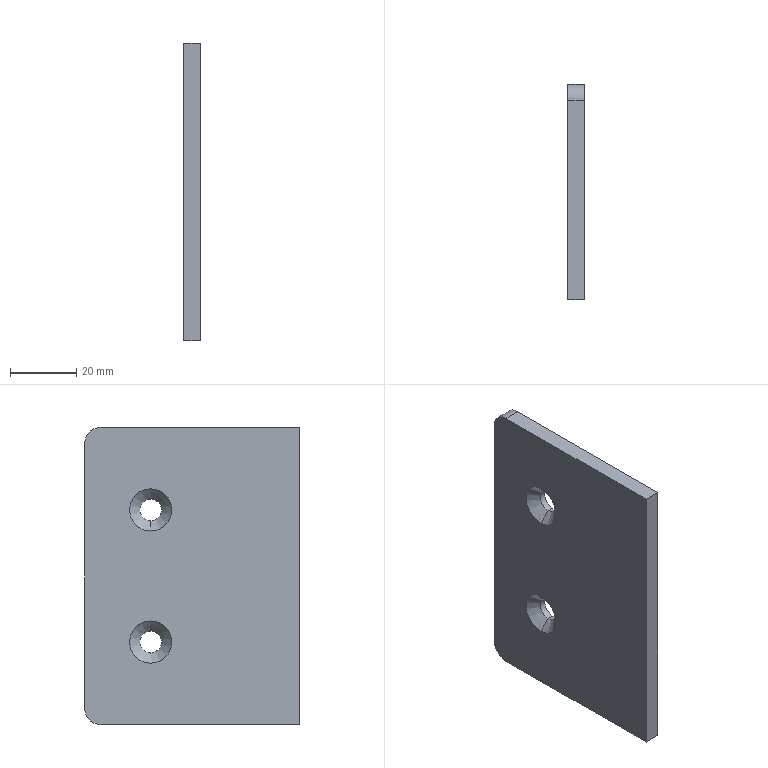Part | SolidWorks | features Extrusion 1, HoleWzd 1 | 1 solid | 16 faces | box 5 x 65 x 90 mm | volume 28593 mm3 | cylinder 6 | plane 6 | cone 4 | commonest cylinder face diameters 6.6 x4 10 x2
STEP:
#1=CARTESIAN_POINT('',(3.1,45.,-23.3));
#2=VERTEX_POINT('',#1);
#3=CARTESIAN_POINT('',(3.1,45.,-16.7));
#4=VERTEX_POINT('',#3);
#5=CARTESIAN_POINT('',(3.1,45.,-20.));
#6=DIRECTION('',(-1.,0.,0.));
#7=DIRECTION('',(0.,0.,1.));
#8=AXIS2_PLACEMENT_3D('',#5,#6,#7);
#9=CIRCLE('',#8,3.3);
#10=EDGE_CURVE('',#2,#4,#9,.T.);
#11=ORIENTED_EDGE('',*,*,#10,.F.);
#12=CARTESIAN_POINT('',(0.,45.,-26.4));
#13=VERTEX_POINT('',#12);
#14=CARTESIAN_POINT('',(0.,45.,-26.4));
#15=DIRECTION('',(-0.7071,0.,-0.7071));
#16=VECTOR('',#15,1000.);
#17=LINE('',#14,#16);
#18=EDGE_CURVE('',#2,#13,#17,.T.);
#19=ORIENTED_EDGE('',*,*,#18,.T.);
#20=CARTESIAN_POINT('',(0.,45.,-13.6));
#21=VERTEX_POINT('',#20);
#22=CARTESIAN_POINT('',(0.,45.,-20.));
#23=DIRECTION('',(-1.,0.,0.));
#24=DIRECTION('',(0.,0.,1.));
#25=AXIS2_PLACEMENT_3D('',#22,#23,#24);
#26=CIRCLE('',#25,6.4);
#27=EDGE_CURVE('',#13,#21,#26,.T.);
#28=ORIENTED_EDGE('',*,*,#27,.T.);
#29=CARTESIAN_POINT('',(0.,45.,-13.6));
#30=DIRECTION('',(-0.7071,0.,0.7071));
#31=VECTOR('',#30,1000.);
#32=LINE('',#29,#31);
#33=EDGE_CURVE('',#4,#21,#32,.T.);
#34=ORIENTED_EDGE('',*,*,#33,.F.);
#35=EDGE_LOOP('',(#11,#19,#28,#34));
#36=FACE_OUTER_BOUND('',#35,.T.);
#37=CARTESIAN_POINT('',(0.,45.,-20.));
#38=DIRECTION('',(-1.,0.,0.));
#39=DIRECTION('',(0.,0.,1.));
#40=AXIS2_PLACEMENT_3D('',#37,#38,#39);
#41=CONICAL_SURFACE('',#40,6.4,0.7854);
#42=ADVANCED_FACE('',(#36),#41,.F.);
#43=CARTESIAN_POINT('',(5.,45.,-23.3));
#44=VERTEX_POINT('',#43);
#45=CARTESIAN_POINT('',(5.,45.,-16.7));
#46=VERTEX_POINT('',#45);
#47=CARTESIAN_POINT('',(5.,45.,-20.));
#48=DIRECTION('',(-1.,0.,0.));
#49=DIRECTION('',(0.,0.,1.));
#50=AXIS2_PLACEMENT_3D('',#47,#48,#49);
#51=CIRCLE('',#50,3.3);
#52=EDGE_CURVE('',#44,#46,#51,.T.);
#53=ORIENTED_EDGE('',*,*,#52,.F.);
#54=CARTESIAN_POINT('',(0.,45.,-23.3));
#55=DIRECTION('',(-1.,0.,0.));
#56=VECTOR('',#55,1000.);
#57=LINE('',#54,#56);
#58=EDGE_CURVE('',#44,#2,#57,.T.);
#59=ORIENTED_EDGE('',*,*,#58,.T.);
#60=ORIENTED_EDGE('',*,*,#10,.T.);
#61=CARTESIAN_POINT('',(0.,45.,-16.7));
#62=DIRECTION('',(-1.,0.,0.));
#63=VECTOR('',#62,1000.);
#64=LINE('',#61,#63);
#65=EDGE_CURVE('',#46,#4,#64,.T.);
#66=ORIENTED_EDGE('',*,*,#65,.F.);
#67=EDGE_LOOP('',(#53,#59,#60,#66));
#68=FACE_OUTER_BOUND('',#67,.T.);
#69=CARTESIAN_POINT('',(0.,45.,-20.));
#70=DIRECTION('',(-1.,0.,0.));
#71=DIRECTION('',(0.,0.,1.));
#72=AXIS2_PLACEMENT_3D('',#69,#70,#71);
#73=CYLINDRICAL_SURFACE('',#72,3.3);
#74=ADVANCED_FACE('',(#68),#73,.F.);
#75=CARTESIAN_POINT('',(3.1,45.,16.7));
#76=VERTEX_POINT('',#75);
#77=CARTESIAN_POINT('',(3.1,45.,23.3));
#78=VERTEX_POINT('',#77);
#79=CARTESIAN_POINT('',(3.1,45.,20.));
#80=DIRECTION('',(-1.,0.,0.));
#81=DIRECTION('',(0.,0.,1.));
#82=AXIS2_PLACEMENT_3D('',#79,#80,#81);
#83=CIRCLE('',#82,3.3);
#84=EDGE_CURVE('',#76,#78,#83,.T.);
#85=ORIENTED_EDGE('',*,*,#84,.F.);
#86=CARTESIAN_POINT('',(0.,45.,13.6));
#87=VERTEX_POINT('',#86);
#88=CARTESIAN_POINT('',(0.,45.,13.6));
#89=DIRECTION('',(-0.7071,0.,-0.7071));
#90=VECTOR('',#89,1000.);
#91=LINE('',#88,#90);
#92=EDGE_CURVE('',#76,#87,#91,.T.);
#93=ORIENTED_EDGE('',*,*,#92,.T.);
#94=CARTESIAN_POINT('',(0.,45.,26.4));
#95=VERTEX_POINT('',#94);
#96=CARTESIAN_POINT('',(0.,45.,20.));
#97=DIRECTION('',(-1.,0.,0.));
#98=DIRECTION('',(0.,0.,1.));
#99=AXIS2_PLACEMENT_3D('',#96,#97,#98);
#100=CIRCLE('',#99,6.4);
#101=EDGE_CURVE('',#87,#95,#100,.T.);
#102=ORIENTED_EDGE('',*,*,#101,.T.);
#103=CARTESIAN_POINT('',(0.,45.,26.4));
#104=DIRECTION('',(-0.7071,0.,0.7071));
#105=VECTOR('',#104,1000.);
#106=LINE('',#103,#105);
#107=EDGE_CURVE('',#78,#95,#106,.T.);
#108=ORIENTED_EDGE('',*,*,#107,.F.);
#109=EDGE_LOOP('',(#85,#93,#102,#108));
#110=FACE_OUTER_BOUND('',#109,.T.);
#111=CARTESIAN_POINT('',(0.,45.,20.));
#112=DIRECTION('',(-1.,0.,0.));
#113=DIRECTION('',(0.,0.,1.));
#114=AXIS2_PLACEMENT_3D('',#111,#112,#113);
#115=CONICAL_SURFACE('',#114,6.4,0.7854);
#116=ADVANCED_FACE('',(#110),#115,.F.);
#117=CARTESIAN_POINT('',(5.,45.,16.7));
#118=VERTEX_POINT('',#117);
#119=CARTESIAN_POINT('',(5.,45.,23.3));
#120=VERTEX_POINT('',#119);
#121=CARTESIAN_POINT('',(5.,45.,20.));
#122=DIRECTION('',(-1.,0.,0.));
#123=DIRECTION('',(0.,0.,1.));
#124=AXIS2_PLACEMENT_3D('',#121,#122,#123);
#125=CIRCLE('',#124,3.3);
#126=EDGE_CURVE('',#118,#120,#125,.T.);
#127=ORIENTED_EDGE('',*,*,#126,.F.);
#128=CARTESIAN_POINT('',(0.,45.,16.7));
#129=DIRECTION('',(-1.,0.,0.));
#130=VECTOR('',#129,1000.);
#131=LINE('',#128,#130);
#132=EDGE_CURVE('',#118,#76,#131,.T.);
#133=ORIENTED_EDGE('',*,*,#132,.T.);
#134=ORIENTED_EDGE('',*,*,#84,.T.);
#135=CARTESIAN_POINT('',(0.,45.,23.3));
#136=DIRECTION('',(-1.,0.,0.));
#137=VECTOR('',#136,1000.);
#138=LINE('',#135,#137);
#139=EDGE_CURVE('',#120,#78,#138,.T.);
#140=ORIENTED_EDGE('',*,*,#139,.F.);
#141=EDGE_LOOP('',(#127,#133,#134,#140));
#142=FACE_OUTER_BOUND('',#141,.T.);
#143=CARTESIAN_POINT('',(0.,45.,20.));
#144=DIRECTION('',(-1.,0.,0.));
#145=DIRECTION('',(0.,0.,1.));
#146=AXIS2_PLACEMENT_3D('',#143,#144,#145);
#147=CYLINDRICAL_SURFACE('',#146,3.3);
#148=ADVANCED_FACE('',(#142),#147,.F.);
#149=CARTESIAN_POINT('',(0.,65.,40.));
#150=VERTEX_POINT('',#149);
#151=CARTESIAN_POINT('',(0.,60.,45.));
#152=VERTEX_POINT('',#151);
#153=CARTESIAN_POINT('',(0.,60.,40.));
#154=DIRECTION('',(1.,0.,0.));
#155=DIRECTION('',(0.,0.,-1.));
#156=AXIS2_PLACEMENT_3D('',#153,#154,#155);
#157=CIRCLE('',#156,5.);
#158=EDGE_CURVE('',#150,#152,#157,.T.);
#159=ORIENTED_EDGE('',*,*,#158,.T.);
#160=CARTESIAN_POINT('',(5.,60.,45.));
#161=VERTEX_POINT('',#160);
#162=CARTESIAN_POINT('',(5.,60.,45.));
#163=DIRECTION('',(-1.,0.,0.));
#164=VECTOR('',#163,1000.);
#165=LINE('',#162,#164);
#166=EDGE_CURVE('',#161,#152,#165,.T.);
#167=ORIENTED_EDGE('',*,*,#166,.F.);
#168=CARTESIAN_POINT('',(5.,65.,40.));
#169=VERTEX_POINT('',#168);
#170=CARTESIAN_POINT('',(5.,60.,40.));
#171=DIRECTION('',(1.,0.,0.));
#172=DIRECTION('',(0.,0.,-1.));
#173=AXIS2_PLACEMENT_3D('',#170,#171,#172);
#174=CIRCLE('',#173,5.);
#175=EDGE_CURVE('',#169,#161,#174,.T.);
#176=ORIENTED_EDGE('',*,*,#175,.F.);
#177=CARTESIAN_POINT('',(5.,65.,40.));
#178=DIRECTION('',(-1.,0.,0.));
#179=VECTOR('',#178,1000.);
#180=LINE('',#177,#179);
#181=EDGE_CURVE('',#169,#150,#180,.T.);
#182=ORIENTED_EDGE('',*,*,#181,.T.);
#183=EDGE_LOOP('',(#159,#167,#176,#182));
#184=FACE_OUTER_BOUND('',#183,.T.);
#185=CARTESIAN_POINT('',(5.,60.,40.));
#186=DIRECTION('',(-1.,0.,0.));
#187=DIRECTION('',(0.,0.,1.));
#188=AXIS2_PLACEMENT_3D('',#185,#186,#187);
#189=CYLINDRICAL_SURFACE('',#188,5.);
#190=ADVANCED_FACE('',(#184),#189,.T.);
#191=CARTESIAN_POINT('',(0.,0.,45.));
#192=VERTEX_POINT('',#191);
#193=CARTESIAN_POINT('',(0.,60.,45.));
#194=DIRECTION('',(0.,-1.,0.));
#195=VECTOR('',#194,1000.);
#196=LINE('',#193,#195);
#197=EDGE_CURVE('',#152,#192,#196,.T.);
#198=ORIENTED_EDGE('',*,*,#197,.T.);
#199=CARTESIAN_POINT('',(5.,0.,45.));
#200=VERTEX_POINT('',#199);
#201=CARTESIAN_POINT('',(5.,0.,45.));
#202=DIRECTION('',(-1.,0.,0.));
#203=VECTOR('',#202,1000.);
#204=LINE('',#201,#203);
#205=EDGE_CURVE('',#200,#192,#204,.T.);
#206=ORIENTED_EDGE('',*,*,#205,.F.);
#207=CARTESIAN_POINT('',(5.,60.,45.));
#208=DIRECTION('',(0.,-1.,0.));
#209=VECTOR('',#208,1000.);
#210=LINE('',#207,#209);
#211=EDGE_CURVE('',#161,#200,#210,.T.);
#212=ORIENTED_EDGE('',*,*,#211,.F.);
#213=ORIENTED_EDGE('',*,*,#166,.T.);
#214=EDGE_LOOP('',(#198,#206,#212,#213));
#215=FACE_OUTER_BOUND('',#214,.T.);
#216=CARTESIAN_POINT('',(5.,60.,45.));
#217=DIRECTION('',(0.,0.,-1.));
#218=DIRECTION('',(0.,1.,0.));
#219=AXIS2_PLACEMENT_3D('',#216,#217,#218);
#220=PLANE('',#219);
#221=ADVANCED_FACE('',(#215),#220,.F.);
#222=CARTESIAN_POINT('',(0.,0.,-45.));
#223=VERTEX_POINT('',#222);
#224=CARTESIAN_POINT('',(0.,0.,45.));
#225=DIRECTION('',(0.,0.,-1.));
#226=VECTOR('',#225,1000.);
#227=LINE('',#224,#226);
#228=EDGE_CURVE('',#192,#223,#227,.T.);
#229=ORIENTED_EDGE('',*,*,#228,.T.);
#230=CARTESIAN_POINT('',(5.,0.,-45.));
#231=VERTEX_POINT('',#230);
#232=CARTESIAN_POINT('',(5.,0.,-45.));
#233=DIRECTION('',(-1.,0.,0.));
#234=VECTOR('',#233,1000.);
#235=LINE('',#232,#234);
#236=EDGE_CURVE('',#231,#223,#235,.T.);
#237=ORIENTED_EDGE('',*,*,#236,.F.);
#238=CARTESIAN_POINT('',(5.,0.,45.));
#239=DIRECTION('',(0.,0.,-1.));
#240=VECTOR('',#239,1000.);
#241=LINE('',#238,#240);
#242=EDGE_CURVE('',#200,#231,#241,.T.);
#243=ORIENTED_EDGE('',*,*,#242,.F.);
#244=ORIENTED_EDGE('',*,*,#205,.T.);
#245=EDGE_LOOP('',(#229,#237,#243,#244));
#246=FACE_OUTER_BOUND('',#245,.T.);
#247=CARTESIAN_POINT('',(5.,0.,45.));
#248=DIRECTION('',(0.,1.,0.));
#249=DIRECTION('',(0.,0.,1.));
#250=AXIS2_PLACEMENT_3D('',#247,#248,#249);
#251=PLANE('',#250);
#252=ADVANCED_FACE('',(#246),#251,.F.);
#253=CARTESIAN_POINT('',(0.,60.,-45.));
#254=VERTEX_POINT('',#253);
#255=CARTESIAN_POINT('',(0.,0.,-45.));
#256=DIRECTION('',(0.,1.,0.));
#257=VECTOR('',#256,1000.);
#258=LINE('',#255,#257);
#259=EDGE_CURVE('',#223,#254,#258,.T.);
#260=ORIENTED_EDGE('',*,*,#259,.T.);
#261=CARTESIAN_POINT('',(5.,60.,-45.));
#262=VERTEX_POINT('',#261);
#263=CARTESIAN_POINT('',(5.,60.,-45.));
#264=DIRECTION('',(-1.,0.,0.));
#265=VECTOR('',#264,1000.);
#266=LINE('',#263,#265);
#267=EDGE_CURVE('',#262,#254,#266,.T.);
#268=ORIENTED_EDGE('',*,*,#267,.F.);
#269=CARTESIAN_POINT('',(5.,0.,-45.));
#270=DIRECTION('',(0.,1.,0.));
#271=VECTOR('',#270,1000.);
#272=LINE('',#269,#271);
#273=EDGE_CURVE('',#231,#262,#272,.T.);
#274=ORIENTED_EDGE('',*,*,#273,.F.);
#275=ORIENTED_EDGE('',*,*,#236,.T.);
#276=EDGE_LOOP('',(#260,#268,#274,#275));
#277=FACE_OUTER_BOUND('',#276,.T.);
#278=CARTESIAN_POINT('',(5.,0.,-45.));
#279=DIRECTION('',(0.,0.,1.));
#280=DIRECTION('',(0.,-1.,0.));
#281=AXIS2_PLACEMENT_3D('',#278,#279,#280);
#282=PLANE('',#281);
#283=ADVANCED_FACE('',(#277),#282,.F.);
#284=CARTESIAN_POINT('',(0.,65.,-40.));
#285=VERTEX_POINT('',#284);
#286=CARTESIAN_POINT('',(0.,60.,-40.));
#287=DIRECTION('',(1.,0.,0.));
#288=DIRECTION('',(0.,0.,-1.));
#289=AXIS2_PLACEMENT_3D('',#286,#287,#288);
#290=CIRCLE('',#289,5.);
#291=EDGE_CURVE('',#254,#285,#290,.T.);
#292=ORIENTED_EDGE('',*,*,#291,.T.);
#293=CARTESIAN_POINT('',(5.,65.,-40.));
#294=VERTEX_POINT('',#293);
#295=CARTESIAN_POINT('',(5.,65.,-40.));
#296=DIRECTION('',(-1.,0.,0.));
#297=VECTOR('',#296,1000.);
#298=LINE('',#295,#297);
#299=EDGE_CURVE('',#294,#285,#298,.T.);
#300=ORIENTED_EDGE('',*,*,#299,.F.);
#301=CARTESIAN_POINT('',(5.,60.,-40.));
#302=DIRECTION('',(1.,0.,0.));
#303=DIRECTION('',(0.,0.,-1.));
#304=AXIS2_PLACEMENT_3D('',#301,#302,#303);
#305=CIRCLE('',#304,5.);
#306=EDGE_CURVE('',#262,#294,#305,.T.);
#307=ORIENTED_EDGE('',*,*,#306,.F.);
#308=ORIENTED_EDGE('',*,*,#267,.T.);
#309=EDGE_LOOP('',(#292,#300,#307,#308));
#310=FACE_OUTER_BOUND('',#309,.T.);
#311=CARTESIAN_POINT('',(5.,60.,-40.));
#312=DIRECTION('',(-1.,0.,0.));
#313=DIRECTION('',(0.,0.,1.));
#314=AXIS2_PLACEMENT_3D('',#311,#312,#313);
#315=CYLINDRICAL_SURFACE('',#314,5.);
#316=ADVANCED_FACE('',(#310),#315,.T.);
#317=CARTESIAN_POINT('',(0.,65.,-40.));
#318=DIRECTION('',(0.,0.,1.));
#319=VECTOR('',#318,1000.);
#320=LINE('',#317,#319);
#321=EDGE_CURVE('',#285,#150,#320,.T.);
#322=ORIENTED_EDGE('',*,*,#321,.T.);
#323=ORIENTED_EDGE('',*,*,#181,.F.);
#324=CARTESIAN_POINT('',(5.,65.,-40.));
#325=DIRECTION('',(0.,0.,1.));
#326=VECTOR('',#325,1000.);
#327=LINE('',#324,#326);
#328=EDGE_CURVE('',#294,#169,#327,.T.);
#329=ORIENTED_EDGE('',*,*,#328,.F.);
#330=ORIENTED_EDGE('',*,*,#299,.T.);
#331=EDGE_LOOP('',(#322,#323,#329,#330));
#332=FACE_OUTER_BOUND('',#331,.T.);
#333=CARTESIAN_POINT('',(5.,65.,-40.));
#334=DIRECTION('',(0.,-1.,0.));
#335=DIRECTION('',(0.,0.,-1.));
#336=AXIS2_PLACEMENT_3D('',#333,#334,#335);
#337=PLANE('',#336);
#338=ADVANCED_FACE('',(#332),#337,.F.);
#339=CARTESIAN_POINT('',(5.,45.,-20.));
#340=DIRECTION('',(-1.,0.,0.));
#341=DIRECTION('',(0.,0.,1.));
#342=AXIS2_PLACEMENT_3D('',#339,#340,#341);
#343=CIRCLE('',#342,3.3);
#344=EDGE_CURVE('',#46,#44,#343,.T.);
#345=ORIENTED_EDGE('',*,*,#344,.T.);
#346=ORIENTED_EDGE('',*,*,#52,.T.);
#347=EDGE_LOOP('',(#345,#346));
#348=FACE_BOUND('',#347,.T.);
#349=CARTESIAN_POINT('',(5.,45.,20.));
#350=DIRECTION('',(-1.,0.,0.));
#351=DIRECTION('',(0.,0.,1.));
#352=AXIS2_PLACEMENT_3D('',#349,#350,#351);
#353=CIRCLE('',#352,3.3);
#354=EDGE_CURVE('',#120,#118,#353,.T.);
#355=ORIENTED_EDGE('',*,*,#354,.T.);
#356=ORIENTED_EDGE('',*,*,#126,.T.);
#357=EDGE_LOOP('',(#355,#356));
#358=FACE_BOUND('',#357,.T.);
#359=ORIENTED_EDGE('',*,*,#175,.T.);
#360=ORIENTED_EDGE('',*,*,#211,.T.);
#361=ORIENTED_EDGE('',*,*,#242,.T.);
#362=ORIENTED_EDGE('',*,*,#273,.T.);
#363=ORIENTED_EDGE('',*,*,#306,.T.);
#364=ORIENTED_EDGE('',*,*,#328,.T.);
#365=EDGE_LOOP('',(#359,#360,#361,#362,#363,#364));
#366=FACE_OUTER_BOUND('',#365,.T.);
#367=CARTESIAN_POINT('',(5.,60.,40.));
#368=DIRECTION('',(1.,0.,0.));
#369=DIRECTION('',(0.,0.,-1.));
#370=AXIS2_PLACEMENT_3D('',#367,#368,#369);
#371=PLANE('',#370);
#372=ADVANCED_FACE('',(#348,#358,#366),#371,.T.);
#373=CARTESIAN_POINT('',(0.,45.,-20.));
#374=DIRECTION('',(-1.,0.,0.));
#375=DIRECTION('',(0.,0.,1.));
#376=AXIS2_PLACEMENT_3D('',#373,#374,#375);
#377=CIRCLE('',#376,6.4);
#378=EDGE_CURVE('',#21,#13,#377,.T.);
#379=ORIENTED_EDGE('',*,*,#378,.F.);
#380=ORIENTED_EDGE('',*,*,#27,.F.);
#381=EDGE_LOOP('',(#379,#380));
#382=FACE_BOUND('',#381,.T.);
#383=CARTESIAN_POINT('',(0.,45.,20.));
#384=DIRECTION('',(-1.,0.,0.));
#385=DIRECTION('',(0.,0.,1.));
#386=AXIS2_PLACEMENT_3D('',#383,#384,#385);
#387=CIRCLE('',#386,6.4);
#388=EDGE_CURVE('',#95,#87,#387,.T.);
#389=ORIENTED_EDGE('',*,*,#388,.F.);
#390=ORIENTED_EDGE('',*,*,#101,.F.);
#391=EDGE_LOOP('',(#389,#390));
#392=FACE_BOUND('',#391,.T.);
#393=ORIENTED_EDGE('',*,*,#158,.F.);
#394=ORIENTED_EDGE('',*,*,#321,.F.);
#395=ORIENTED_EDGE('',*,*,#291,.F.);
#396=ORIENTED_EDGE('',*,*,#259,.F.);
#397=ORIENTED_EDGE('',*,*,#228,.F.);
#398=ORIENTED_EDGE('',*,*,#197,.F.);
#399=EDGE_LOOP('',(#393,#394,#395,#396,#397,#398));
#400=FACE_OUTER_BOUND('',#399,.T.);
#401=CARTESIAN_POINT('',(0.,60.,40.));
#402=DIRECTION('',(1.,0.,0.));
#403=DIRECTION('',(0.,0.,-1.));
#404=AXIS2_PLACEMENT_3D('',#401,#402,#403);
#405=PLANE('',#404);
#406=ADVANCED_FACE('',(#382,#392,#400),#405,.F.);
#407=ORIENTED_EDGE('',*,*,#132,.F.);
#408=ORIENTED_EDGE('',*,*,#354,.F.);
#409=ORIENTED_EDGE('',*,*,#139,.T.);
#410=CARTESIAN_POINT('',(3.1,45.,20.));
#411=DIRECTION('',(-1.,0.,0.));
#412=DIRECTION('',(0.,0.,1.));
#413=AXIS2_PLACEMENT_3D('',#410,#411,#412);
#414=CIRCLE('',#413,3.3);
#415=EDGE_CURVE('',#78,#76,#414,.T.);
#416=ORIENTED_EDGE('',*,*,#415,.T.);
#417=EDGE_LOOP('',(#407,#408,#409,#416));
#418=FACE_OUTER_BOUND('',#417,.T.);
#419=CARTESIAN_POINT('',(0.,45.,20.));
#420=DIRECTION('',(-1.,0.,0.));
#421=DIRECTION('',(0.,0.,1.));
#422=AXIS2_PLACEMENT_3D('',#419,#420,#421);
#423=CYLINDRICAL_SURFACE('',#422,3.3);
#424=ADVANCED_FACE('',(#418),#423,.F.);
#425=ORIENTED_EDGE('',*,*,#92,.F.);
#426=ORIENTED_EDGE('',*,*,#415,.F.);
#427=ORIENTED_EDGE('',*,*,#107,.T.);
#428=ORIENTED_EDGE('',*,*,#388,.T.);
#429=EDGE_LOOP('',(#425,#426,#427,#428));
#430=FACE_OUTER_BOUND('',#429,.T.);
#431=CARTESIAN_POINT('',(0.,45.,20.));
#432=DIRECTION('',(-1.,0.,0.));
#433=DIRECTION('',(0.,0.,1.));
#434=AXIS2_PLACEMENT_3D('',#431,#432,#433);
#435=CONICAL_SURFACE('',#434,6.4,0.7854);
#436=ADVANCED_FACE('',(#430),#435,.F.);
#437=ORIENTED_EDGE('',*,*,#58,.F.);
#438=ORIENTED_EDGE('',*,*,#344,.F.);
#439=ORIENTED_EDGE('',*,*,#65,.T.);
#440=CARTESIAN_POINT('',(3.1,45.,-20.));
#441=DIRECTION('',(-1.,0.,0.));
#442=DIRECTION('',(0.,0.,1.));
#443=AXIS2_PLACEMENT_3D('',#440,#441,#442);
#444=CIRCLE('',#443,3.3);
#445=EDGE_CURVE('',#4,#2,#444,.T.);
#446=ORIENTED_EDGE('',*,*,#445,.T.);
#447=EDGE_LOOP('',(#437,#438,#439,#446));
#448=FACE_OUTER_BOUND('',#447,.T.);
#449=CARTESIAN_POINT('',(0.,45.,-20.));
#450=DIRECTION('',(-1.,0.,0.));
#451=DIRECTION('',(0.,0.,1.));
#452=AXIS2_PLACEMENT_3D('',#449,#450,#451);
#453=CYLINDRICAL_SURFACE('',#452,3.3);
#454=ADVANCED_FACE('',(#448),#453,.F.);
#455=ORIENTED_EDGE('',*,*,#18,.F.);
#456=ORIENTED_EDGE('',*,*,#445,.F.);
#457=ORIENTED_EDGE('',*,*,#33,.T.);
#458=ORIENTED_EDGE('',*,*,#378,.T.);
#459=EDGE_LOOP('',(#455,#456,#457,#458));
#460=FACE_OUTER_BOUND('',#459,.T.);
#461=CARTESIAN_POINT('',(0.,45.,-20.));
#462=DIRECTION('',(-1.,0.,0.));
#463=DIRECTION('',(0.,0.,1.));
#464=AXIS2_PLACEMENT_3D('',#461,#462,#463);
#465=CONICAL_SURFACE('',#464,6.4,0.7854);
#466=ADVANCED_FACE('',(#460),#465,.F.);
#467=CLOSED_SHELL('',(#42,#74,#116,#148,#190,#221,#252,#283,#316,#338,#372,#406,#424,#436,#454,#466));
#468=MANIFOLD_SOLID_BREP('',#467);
#469=CARTESIAN_POINT('',(0.,0.,0.));
#470=DIRECTION('',(0.,0.,1.));
#471=DIRECTION('',(1.,0.,0.));
#472=AXIS2_PLACEMENT_3D('',#469,#470,#471);
#473=(LENGTH_UNIT()NAMED_UNIT(*)SI_UNIT(.MILLI.,.METRE.));
#474=UNCERTAINTY_MEASURE_WITH_UNIT(LENGTH_MEASURE(0.00001),#473,'','');
#475=(NAMED_UNIT(*)PLANE_ANGLE_UNIT()SI_UNIT($,.RADIAN.));
#476=(NAMED_UNIT(*)SI_UNIT($,.STERADIAN.)SOLID_ANGLE_UNIT());
#477=(GEOMETRIC_REPRESENTATION_CONTEXT(3)GLOBAL_UNCERTAINTY_ASSIGNED_CONTEXT((#474))GLOBAL_UNIT_ASSIGNED_CONTEXT((#473,#475,#476))REPRESENTATION_CONTEXT('',''));
#478=ADVANCED_BREP_SHAPE_REPRESENTATION('',(#468,#472),#477);